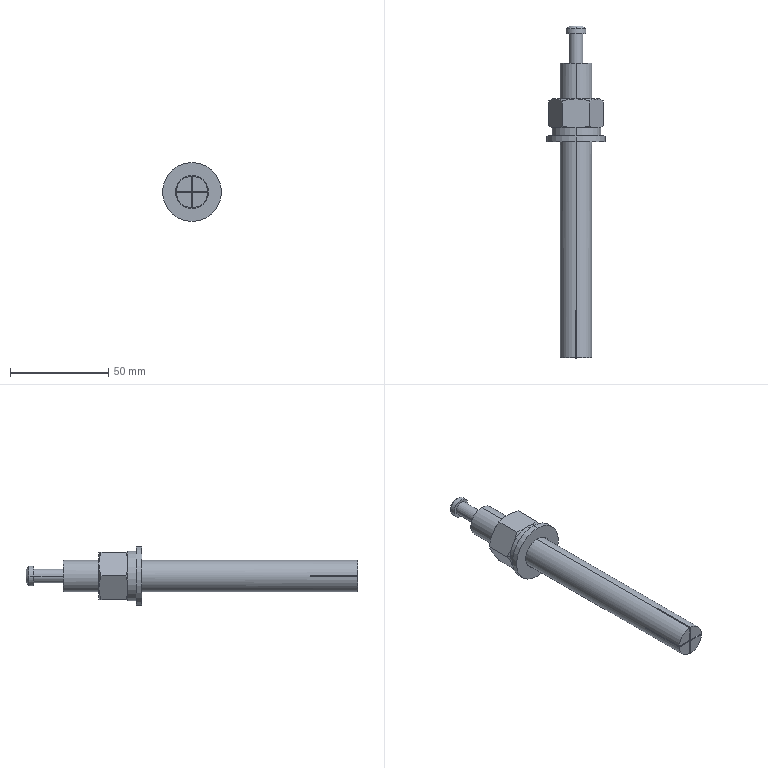Part | STEP file | 5 solids | 64 faces | box 30 x 169 x 30 mm | volume 37532 mm3 | plane 31 | cylinder 18 | cone 15 | commonest cylinder face diameters 16 x4 16.9 x3 25.1 x3 7 x2 10 x2 17 x2